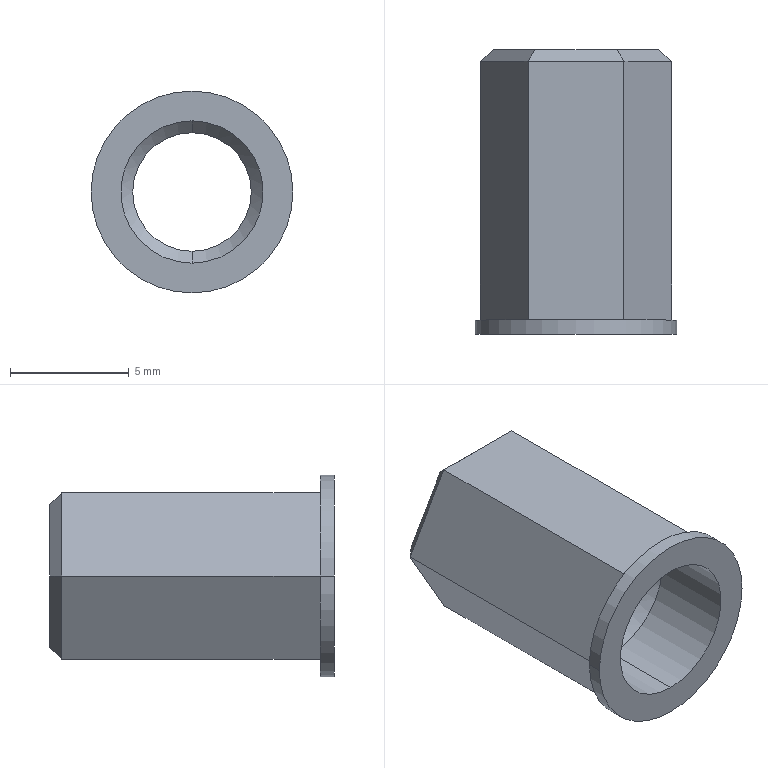Part | SolidWorks | features BaseBody 1 | 1 solid | 23 faces | box 8.5 x 12 x 8.5 mm | volume 246.97 mm3 | plane 15 | cylinder 6 | cone 2 | commonest cylinder face diameters 5 x2 6 x2 8.5 x2
STEP:
#1=CARTESIAN_POINT('',(0.,0.,-3.));
#2=VERTEX_POINT('',#1);
#3=CARTESIAN_POINT('',(0.,0.,3.));
#4=VERTEX_POINT('',#3);
#5=CARTESIAN_POINT('',(0.,0.,0.));
#6=DIRECTION('',(0.,-1.,0.));
#7=DIRECTION('',(0.,0.,-1.));
#8=AXIS2_PLACEMENT_3D('',#5,#6,#7);
#9=CIRCLE('',#8,3.);
#10=EDGE_CURVE('',#2,#4,#9,.T.);
#11=ORIENTED_EDGE('',*,*,#10,.F.);
#12=CARTESIAN_POINT('',(0.,0.,0.));
#13=DIRECTION('',(0.,-1.,0.));
#14=DIRECTION('',(0.,0.,1.));
#15=AXIS2_PLACEMENT_3D('',#12,#13,#14);
#16=CIRCLE('',#15,3.);
#17=EDGE_CURVE('',#4,#2,#16,.T.);
#18=ORIENTED_EDGE('',*,*,#17,.F.);
#19=EDGE_LOOP('',(#11,#18));
#20=FACE_BOUND('',#19,.T.);
#21=CARTESIAN_POINT('',(4.25,0.,0.));
#22=VERTEX_POINT('',#21);
#23=CARTESIAN_POINT('',(-4.25,0.,0.));
#24=VERTEX_POINT('',#23);
#25=CARTESIAN_POINT('',(0.,0.,0.));
#26=DIRECTION('',(0.,-1.,0.));
#27=DIRECTION('',(1.,0.,0.));
#28=AXIS2_PLACEMENT_3D('',#25,#26,#27);
#29=CIRCLE('',#28,4.25);
#30=EDGE_CURVE('',#22,#24,#29,.T.);
#31=ORIENTED_EDGE('',*,*,#30,.T.);
#32=CARTESIAN_POINT('',(0.,0.,0.));
#33=DIRECTION('',(0.,-1.,0.));
#34=DIRECTION('',(-1.,0.,0.));
#35=AXIS2_PLACEMENT_3D('',#32,#33,#34);
#36=CIRCLE('',#35,4.25);
#37=EDGE_CURVE('',#24,#22,#36,.T.);
#38=ORIENTED_EDGE('',*,*,#37,.T.);
#39=EDGE_LOOP('',(#31,#38));
#40=FACE_OUTER_BOUND('',#39,.T.);
#41=CARTESIAN_POINT('',(0.,0.,0.));
#42=DIRECTION('',(0.,1.,0.));
#43=DIRECTION('',(1.,0.,0.));
#44=AXIS2_PLACEMENT_3D('',#41,#42,#43);
#45=PLANE('',#44);
#46=ADVANCED_FACE('',(#20,#40),#45,.F.);
#47=CARTESIAN_POINT('',(-4.25,0.6,0.));
#48=VERTEX_POINT('',#47);
#49=CARTESIAN_POINT('',(-4.25,0.,0.));
#50=DIRECTION('',(0.,1.,0.));
#51=VECTOR('',#50,1000.);
#52=LINE('',#49,#51);
#53=EDGE_CURVE('',#24,#48,#52,.T.);
#54=ORIENTED_EDGE('',*,*,#53,.T.);
#55=CARTESIAN_POINT('',(4.25,0.6,0.));
#56=VERTEX_POINT('',#55);
#57=CARTESIAN_POINT('',(0.,0.6,0.));
#58=DIRECTION('',(0.,-1.,0.));
#59=DIRECTION('',(-1.,0.,0.));
#60=AXIS2_PLACEMENT_3D('',#57,#58,#59);
#61=CIRCLE('',#60,4.25);
#62=EDGE_CURVE('',#48,#56,#61,.T.);
#63=ORIENTED_EDGE('',*,*,#62,.T.);
#64=CARTESIAN_POINT('',(4.25,0.,0.));
#65=DIRECTION('',(0.,1.,0.));
#66=VECTOR('',#65,1000.);
#67=LINE('',#64,#66);
#68=EDGE_CURVE('',#22,#56,#67,.T.);
#69=ORIENTED_EDGE('',*,*,#68,.F.);
#70=ORIENTED_EDGE('',*,*,#37,.F.);
#71=EDGE_LOOP('',(#54,#63,#69,#70));
#72=FACE_OUTER_BOUND('',#71,.T.);
#73=CARTESIAN_POINT('',(0.,0.,0.));
#74=DIRECTION('',(0.,-1.,0.));
#75=DIRECTION('',(-1.,0.,0.));
#76=AXIS2_PLACEMENT_3D('',#73,#74,#75);
#77=CYLINDRICAL_SURFACE('',#76,4.25);
#78=ADVANCED_FACE('',(#72),#77,.T.);
#79=ORIENTED_EDGE('',*,*,#68,.T.);
#80=CARTESIAN_POINT('',(0.,0.6,0.));
#81=DIRECTION('',(0.,-1.,0.));
#82=DIRECTION('',(1.,0.,0.));
#83=AXIS2_PLACEMENT_3D('',#80,#81,#82);
#84=CIRCLE('',#83,4.25);
#85=EDGE_CURVE('',#56,#48,#84,.T.);
#86=ORIENTED_EDGE('',*,*,#85,.T.);
#87=ORIENTED_EDGE('',*,*,#53,.F.);
#88=ORIENTED_EDGE('',*,*,#30,.F.);
#89=EDGE_LOOP('',(#79,#86,#87,#88));
#90=FACE_OUTER_BOUND('',#89,.T.);
#91=CARTESIAN_POINT('',(0.,0.,0.));
#92=DIRECTION('',(0.,-1.,0.));
#93=DIRECTION('',(-1.,0.,0.));
#94=AXIS2_PLACEMENT_3D('',#91,#92,#93);
#95=CYLINDRICAL_SURFACE('',#94,4.25);
#96=ADVANCED_FACE('',(#90),#95,.T.);
#97=CARTESIAN_POINT('',(2.021,0.6,-3.5));
#98=VERTEX_POINT('',#97);
#99=CARTESIAN_POINT('',(-2.021,0.6,-3.5));
#100=VERTEX_POINT('',#99);
#101=CARTESIAN_POINT('',(2.021,0.6,-3.5));
#102=DIRECTION('',(-1.,0.,0.));
#103=VECTOR('',#102,1000.);
#104=LINE('',#101,#103);
#105=EDGE_CURVE('',#98,#100,#104,.T.);
#106=ORIENTED_EDGE('',*,*,#105,.F.);
#107=CARTESIAN_POINT('',(4.041,0.6,0.));
#108=VERTEX_POINT('',#107);
#109=CARTESIAN_POINT('',(4.041,0.6,0.));
#110=DIRECTION('',(-0.5,0.,-0.866));
#111=VECTOR('',#110,1000.);
#112=LINE('',#109,#111);
#113=EDGE_CURVE('',#108,#98,#112,.T.);
#114=ORIENTED_EDGE('',*,*,#113,.F.);
#115=CARTESIAN_POINT('',(2.021,0.6,3.5));
#116=VERTEX_POINT('',#115);
#117=CARTESIAN_POINT('',(2.021,0.6,3.5));
#118=DIRECTION('',(0.5,0.,-0.866));
#119=VECTOR('',#118,1000.);
#120=LINE('',#117,#119);
#121=EDGE_CURVE('',#116,#108,#120,.T.);
#122=ORIENTED_EDGE('',*,*,#121,.F.);
#123=CARTESIAN_POINT('',(-2.021,0.6,3.5));
#124=VERTEX_POINT('',#123);
#125=CARTESIAN_POINT('',(-2.021,0.6,3.5));
#126=DIRECTION('',(1.,0.,0.));
#127=VECTOR('',#126,1000.);
#128=LINE('',#125,#127);
#129=EDGE_CURVE('',#124,#116,#128,.T.);
#130=ORIENTED_EDGE('',*,*,#129,.F.);
#131=CARTESIAN_POINT('',(-4.041,0.6,0.));
#132=VERTEX_POINT('',#131);
#133=CARTESIAN_POINT('',(-4.041,0.6,0.));
#134=DIRECTION('',(0.5,0.,0.866));
#135=VECTOR('',#134,1000.);
#136=LINE('',#133,#135);
#137=EDGE_CURVE('',#132,#124,#136,.T.);
#138=ORIENTED_EDGE('',*,*,#137,.F.);
#139=CARTESIAN_POINT('',(-2.021,0.6,-3.5));
#140=DIRECTION('',(-0.5,0.,0.866));
#141=VECTOR('',#140,1000.);
#142=LINE('',#139,#141);
#143=EDGE_CURVE('',#100,#132,#142,.T.);
#144=ORIENTED_EDGE('',*,*,#143,.F.);
#145=EDGE_LOOP('',(#106,#114,#122,#130,#138,#144));
#146=FACE_BOUND('',#145,.T.);
#147=ORIENTED_EDGE('',*,*,#85,.F.);
#148=ORIENTED_EDGE('',*,*,#62,.F.);
#149=EDGE_LOOP('',(#147,#148));
#150=FACE_OUTER_BOUND('',#149,.T.);
#151=CARTESIAN_POINT('',(0.,0.6,0.));
#152=DIRECTION('',(0.,-1.,0.));
#153=DIRECTION('',(0.,0.,-1.));
#154=AXIS2_PLACEMENT_3D('',#151,#152,#153);
#155=PLANE('',#154);
#156=ADVANCED_FACE('',(#146,#150),#155,.F.);
#157=CARTESIAN_POINT('',(-4.041,11.5,0.));
#158=VERTEX_POINT('',#157);
#159=CARTESIAN_POINT('',(-4.041,0.6,0.));
#160=DIRECTION('',(0.,1.,0.));
#161=VECTOR('',#160,1000.);
#162=LINE('',#159,#161);
#163=EDGE_CURVE('',#132,#158,#162,.T.);
#164=ORIENTED_EDGE('',*,*,#163,.T.);
#165=CARTESIAN_POINT('',(-2.021,11.5,-3.5));
#166=VERTEX_POINT('',#165);
#167=CARTESIAN_POINT('',(-2.021,11.5,-3.5));
#168=DIRECTION('',(-0.5,0.,0.866));
#169=VECTOR('',#168,1000.);
#170=LINE('',#167,#169);
#171=EDGE_CURVE('',#166,#158,#170,.T.);
#172=ORIENTED_EDGE('',*,*,#171,.F.);
#173=CARTESIAN_POINT('',(-2.021,0.6,-3.5));
#174=DIRECTION('',(0.,1.,0.));
#175=VECTOR('',#174,1000.);
#176=LINE('',#173,#175);
#177=EDGE_CURVE('',#100,#166,#176,.T.);
#178=ORIENTED_EDGE('',*,*,#177,.F.);
#179=ORIENTED_EDGE('',*,*,#143,.T.);
#180=EDGE_LOOP('',(#164,#172,#178,#179));
#181=FACE_OUTER_BOUND('',#180,.T.);
#182=CARTESIAN_POINT('',(-2.021,0.,-3.5));
#183=DIRECTION('',(-0.866,0.,-0.5));
#184=DIRECTION('',(-0.5,0.,0.866));
#185=AXIS2_PLACEMENT_3D('',#182,#183,#184);
#186=PLANE('',#185);
#187=ADVANCED_FACE('',(#181),#186,.T.);
#188=ORIENTED_EDGE('',*,*,#177,.T.);
#189=CARTESIAN_POINT('',(2.021,11.5,-3.5));
#190=VERTEX_POINT('',#189);
#191=CARTESIAN_POINT('',(2.021,11.5,-3.5));
#192=DIRECTION('',(-1.,0.,0.));
#193=VECTOR('',#192,1000.);
#194=LINE('',#191,#193);
#195=EDGE_CURVE('',#190,#166,#194,.T.);
#196=ORIENTED_EDGE('',*,*,#195,.F.);
#197=CARTESIAN_POINT('',(2.021,0.6,-3.5));
#198=DIRECTION('',(0.,1.,0.));
#199=VECTOR('',#198,1000.);
#200=LINE('',#197,#199);
#201=EDGE_CURVE('',#98,#190,#200,.T.);
#202=ORIENTED_EDGE('',*,*,#201,.F.);
#203=ORIENTED_EDGE('',*,*,#105,.T.);
#204=EDGE_LOOP('',(#188,#196,#202,#203));
#205=FACE_OUTER_BOUND('',#204,.T.);
#206=CARTESIAN_POINT('',(2.021,0.,-3.5));
#207=DIRECTION('',(0.,0.,-1.));
#208=DIRECTION('',(0.,-1.,0.));
#209=AXIS2_PLACEMENT_3D('',#206,#207,#208);
#210=PLANE('',#209);
#211=ADVANCED_FACE('',(#205),#210,.T.);
#212=ORIENTED_EDGE('',*,*,#201,.T.);
#213=CARTESIAN_POINT('',(4.041,11.5,0.));
#214=VERTEX_POINT('',#213);
#215=CARTESIAN_POINT('',(4.041,11.5,0.));
#216=DIRECTION('',(-0.5,0.,-0.866));
#217=VECTOR('',#216,1000.);
#218=LINE('',#215,#217);
#219=EDGE_CURVE('',#214,#190,#218,.T.);
#220=ORIENTED_EDGE('',*,*,#219,.F.);
#221=CARTESIAN_POINT('',(4.041,0.6,0.));
#222=DIRECTION('',(0.,1.,0.));
#223=VECTOR('',#222,1000.);
#224=LINE('',#221,#223);
#225=EDGE_CURVE('',#108,#214,#224,.T.);
#226=ORIENTED_EDGE('',*,*,#225,.F.);
#227=ORIENTED_EDGE('',*,*,#113,.T.);
#228=EDGE_LOOP('',(#212,#220,#226,#227));
#229=FACE_OUTER_BOUND('',#228,.T.);
#230=CARTESIAN_POINT('',(4.041,0.,0.));
#231=DIRECTION('',(0.866,0.,-0.5));
#232=DIRECTION('',(0.,-1.,0.));
#233=AXIS2_PLACEMENT_3D('',#230,#231,#232);
#234=PLANE('',#233);
#235=ADVANCED_FACE('',(#229),#234,.T.);
#236=ORIENTED_EDGE('',*,*,#225,.T.);
#237=CARTESIAN_POINT('',(2.021,11.5,3.5));
#238=VERTEX_POINT('',#237);
#239=CARTESIAN_POINT('',(2.021,11.5,3.5));
#240=DIRECTION('',(0.5,0.,-0.866));
#241=VECTOR('',#240,1000.);
#242=LINE('',#239,#241);
#243=EDGE_CURVE('',#238,#214,#242,.T.);
#244=ORIENTED_EDGE('',*,*,#243,.F.);
#245=CARTESIAN_POINT('',(2.021,0.6,3.5));
#246=DIRECTION('',(0.,1.,0.));
#247=VECTOR('',#246,1000.);
#248=LINE('',#245,#247);
#249=EDGE_CURVE('',#116,#238,#248,.T.);
#250=ORIENTED_EDGE('',*,*,#249,.F.);
#251=ORIENTED_EDGE('',*,*,#121,.T.);
#252=EDGE_LOOP('',(#236,#244,#250,#251));
#253=FACE_OUTER_BOUND('',#252,.T.);
#254=CARTESIAN_POINT('',(2.021,0.,3.5));
#255=DIRECTION('',(0.866,0.,0.5));
#256=DIRECTION('',(0.,-1.,0.));
#257=AXIS2_PLACEMENT_3D('',#254,#255,#256);
#258=PLANE('',#257);
#259=ADVANCED_FACE('',(#253),#258,.T.);
#260=ORIENTED_EDGE('',*,*,#249,.T.);
#261=CARTESIAN_POINT('',(-2.021,11.5,3.5));
#262=VERTEX_POINT('',#261);
#263=CARTESIAN_POINT('',(-2.021,11.5,3.5));
#264=DIRECTION('',(1.,0.,0.));
#265=VECTOR('',#264,1000.);
#266=LINE('',#263,#265);
#267=EDGE_CURVE('',#262,#238,#266,.T.);
#268=ORIENTED_EDGE('',*,*,#267,.F.);
#269=CARTESIAN_POINT('',(-2.021,0.6,3.5));
#270=DIRECTION('',(0.,1.,0.));
#271=VECTOR('',#270,1000.);
#272=LINE('',#269,#271);
#273=EDGE_CURVE('',#124,#262,#272,.T.);
#274=ORIENTED_EDGE('',*,*,#273,.F.);
#275=ORIENTED_EDGE('',*,*,#129,.T.);
#276=EDGE_LOOP('',(#260,#268,#274,#275));
#277=FACE_OUTER_BOUND('',#276,.T.);
#278=CARTESIAN_POINT('',(-2.021,0.,3.5));
#279=DIRECTION('',(0.,0.,1.));
#280=DIRECTION('',(1.,0.,0.));
#281=AXIS2_PLACEMENT_3D('',#278,#279,#280);
#282=PLANE('',#281);
#283=ADVANCED_FACE('',(#277),#282,.T.);
#284=ORIENTED_EDGE('',*,*,#273,.T.);
#285=CARTESIAN_POINT('',(-4.041,11.5,0.));
#286=DIRECTION('',(0.5,0.,0.866));
#287=VECTOR('',#286,1000.);
#288=LINE('',#285,#287);
#289=EDGE_CURVE('',#158,#262,#288,.T.);
#290=ORIENTED_EDGE('',*,*,#289,.F.);
#291=ORIENTED_EDGE('',*,*,#163,.F.);
#292=ORIENTED_EDGE('',*,*,#137,.T.);
#293=EDGE_LOOP('',(#284,#290,#291,#292));
#294=FACE_OUTER_BOUND('',#293,.T.);
#295=CARTESIAN_POINT('',(-4.041,0.,0.));
#296=DIRECTION('',(-0.866,0.,0.5));
#297=DIRECTION('',(0.,1.,0.));
#298=AXIS2_PLACEMENT_3D('',#295,#296,#297);
#299=PLANE('',#298);
#300=ADVANCED_FACE('',(#294),#299,.T.);
#301=CARTESIAN_POINT('',(-1.732,12.,3.));
#302=VERTEX_POINT('',#301);
#303=CARTESIAN_POINT('',(-2.021,11.5,3.5));
#304=DIRECTION('',(0.378,0.6547,-0.6547));
#305=VECTOR('',#304,1000.);
#306=LINE('',#303,#305);
#307=EDGE_CURVE('',#262,#302,#306,.T.);
#308=ORIENTED_EDGE('',*,*,#307,.T.);
#309=CARTESIAN_POINT('',(-3.464,12.,0.));
#310=VERTEX_POINT('',#309);
#311=CARTESIAN_POINT('',(-3.464,12.,0.));
#312=DIRECTION('',(0.5,0.,0.866));
#313=VECTOR('',#312,1000.);
#314=LINE('',#311,#313);
#315=EDGE_CURVE('',#310,#302,#314,.T.);
#316=ORIENTED_EDGE('',*,*,#315,.F.);
#317=CARTESIAN_POINT('',(-4.041,11.5,0.));
#318=DIRECTION('',(0.7559,0.6547,0.));
#319=VECTOR('',#318,1000.);
#320=LINE('',#317,#319);
#321=EDGE_CURVE('',#158,#310,#320,.T.);
#322=ORIENTED_EDGE('',*,*,#321,.F.);
#323=ORIENTED_EDGE('',*,*,#289,.T.);
#324=EDGE_LOOP('',(#308,#316,#322,#323));
#325=FACE_OUTER_BOUND('',#324,.T.);
#326=CARTESIAN_POINT('',(-2.815,11.75,1.625));
#327=DIRECTION('',(-0.6124,0.7071,0.3536));
#328=DIRECTION('',(0.5,0.,0.866));
#329=AXIS2_PLACEMENT_3D('',#326,#327,#328);
#330=PLANE('',#329);
#331=ADVANCED_FACE('',(#325),#330,.T.);
#332=ORIENTED_EDGE('',*,*,#321,.T.);
#333=CARTESIAN_POINT('',(-1.732,12.,-3.));
#334=VERTEX_POINT('',#333);
#335=CARTESIAN_POINT('',(-1.732,12.,-3.));
#336=DIRECTION('',(-0.5,0.,0.866));
#337=VECTOR('',#336,1000.);
#338=LINE('',#335,#337);
#339=EDGE_CURVE('',#334,#310,#338,.T.);
#340=ORIENTED_EDGE('',*,*,#339,.F.);
#341=CARTESIAN_POINT('',(-2.021,11.5,-3.5));
#342=DIRECTION('',(0.378,0.6547,0.6547));
#343=VECTOR('',#342,1000.);
#344=LINE('',#341,#343);
#345=EDGE_CURVE('',#166,#334,#344,.T.);
#346=ORIENTED_EDGE('',*,*,#345,.F.);
#347=ORIENTED_EDGE('',*,*,#171,.T.);
#348=EDGE_LOOP('',(#332,#340,#346,#347));
#349=FACE_OUTER_BOUND('',#348,.T.);
#350=CARTESIAN_POINT('',(-2.815,11.75,-1.625));
#351=DIRECTION('',(-0.6124,0.7071,-0.3536));
#352=DIRECTION('',(-0.5,0.,0.866));
#353=AXIS2_PLACEMENT_3D('',#350,#351,#352);
#354=PLANE('',#353);
#355=ADVANCED_FACE('',(#349),#354,.T.);
#356=CARTESIAN_POINT('',(1.732,12.,-3.));
#357=VERTEX_POINT('',#356);
#358=CARTESIAN_POINT('',(2.021,11.5,-3.5));
#359=DIRECTION('',(-0.378,0.6547,0.6547));
#360=VECTOR('',#359,1000.);
#361=LINE('',#358,#360);
#362=EDGE_CURVE('',#190,#357,#361,.T.);
#363=ORIENTED_EDGE('',*,*,#362,.F.);
#364=ORIENTED_EDGE('',*,*,#195,.T.);
#365=ORIENTED_EDGE('',*,*,#345,.T.);
#366=CARTESIAN_POINT('',(1.732,12.,-3.));
#367=DIRECTION('',(-1.,0.,0.));
#368=VECTOR('',#367,1000.);
#369=LINE('',#366,#368);
#370=EDGE_CURVE('',#357,#334,#369,.T.);
#371=ORIENTED_EDGE('',*,*,#370,.F.);
#372=EDGE_LOOP('',(#363,#364,#365,#371));
#373=FACE_OUTER_BOUND('',#372,.T.);
#374=CARTESIAN_POINT('',(0.,11.75,-3.25));
#375=DIRECTION('',(0.,0.7071,-0.7071));
#376=DIRECTION('',(-1.,0.,0.));
#377=AXIS2_PLACEMENT_3D('',#374,#375,#376);
#378=PLANE('',#377);
#379=ADVANCED_FACE('',(#373),#378,.T.);
#380=CARTESIAN_POINT('',(-2.5,12.,0.));
#381=VERTEX_POINT('',#380);
#382=CARTESIAN_POINT('',(2.5,12.,0.));
#383=VERTEX_POINT('',#382);
#384=CARTESIAN_POINT('',(0.,12.,0.));
#385=DIRECTION('',(0.,-1.,0.));
#386=DIRECTION('',(-1.,0.,0.));
#387=AXIS2_PLACEMENT_3D('',#384,#385,#386);
#388=CIRCLE('',#387,2.5);
#389=EDGE_CURVE('',#381,#383,#388,.T.);
#390=ORIENTED_EDGE('',*,*,#389,.T.);
#391=CARTESIAN_POINT('',(0.,12.,0.));
#392=DIRECTION('',(0.,-1.,0.));
#393=DIRECTION('',(1.,0.,0.));
#394=AXIS2_PLACEMENT_3D('',#391,#392,#393);
#395=CIRCLE('',#394,2.5);
#396=EDGE_CURVE('',#383,#381,#395,.T.);
#397=ORIENTED_EDGE('',*,*,#396,.T.);
#398=EDGE_LOOP('',(#390,#397));
#399=FACE_BOUND('',#398,.T.);
#400=ORIENTED_EDGE('',*,*,#370,.T.);
#401=ORIENTED_EDGE('',*,*,#339,.T.);
#402=ORIENTED_EDGE('',*,*,#315,.T.);
#403=CARTESIAN_POINT('',(1.732,12.,3.));
#404=VERTEX_POINT('',#403);
#405=CARTESIAN_POINT('',(-1.732,12.,3.));
#406=DIRECTION('',(1.,0.,0.));
#407=VECTOR('',#406,1000.);
#408=LINE('',#405,#407);
#409=EDGE_CURVE('',#302,#404,#408,.T.);
#410=ORIENTED_EDGE('',*,*,#409,.T.);
#411=CARTESIAN_POINT('',(3.464,12.,0.));
#412=VERTEX_POINT('',#411);
#413=CARTESIAN_POINT('',(1.732,12.,3.));
#414=DIRECTION('',(0.5,0.,-0.866));
#415=VECTOR('',#414,1000.);
#416=LINE('',#413,#415);
#417=EDGE_CURVE('',#404,#412,#416,.T.);
#418=ORIENTED_EDGE('',*,*,#417,.T.);
#419=CARTESIAN_POINT('',(3.464,12.,0.));
#420=DIRECTION('',(-0.5,0.,-0.866));
#421=VECTOR('',#420,1000.);
#422=LINE('',#419,#421);
#423=EDGE_CURVE('',#412,#357,#422,.T.);
#424=ORIENTED_EDGE('',*,*,#423,.T.);
#425=EDGE_LOOP('',(#400,#401,#402,#410,#418,#424));
#426=FACE_OUTER_BOUND('',#425,.T.);
#427=CARTESIAN_POINT('',(0.,12.,0.));
#428=DIRECTION('',(0.,1.,0.));
#429=DIRECTION('',(1.,0.,0.));
#430=AXIS2_PLACEMENT_3D('',#427,#428,#429);
#431=PLANE('',#430);
#432=ADVANCED_FACE('',(#399,#426),#431,.T.);
#433=CARTESIAN_POINT('',(-2.5,4.,0.));
#434=VERTEX_POINT('',#433);
#435=CARTESIAN_POINT('',(0.,4.,2.5));
#436=VERTEX_POINT('',#435);
#437=CARTESIAN_POINT('',(0.,4.,0.));
#438=DIRECTION('',(0.,1.,0.));
#439=DIRECTION('',(-1.,0.,0.));
#440=AXIS2_PLACEMENT_3D('',#437,#438,#439);
#441=CIRCLE('',#440,2.5);
#442=EDGE_CURVE('',#434,#436,#441,.T.);
#443=ORIENTED_EDGE('',*,*,#442,.F.);
#444=CARTESIAN_POINT('',(-2.5,4.,0.));
#445=DIRECTION('',(0.,1.,0.));
#446=VECTOR('',#445,1000.);
#447=LINE('',#444,#446);
#448=EDGE_CURVE('',#434,#381,#447,.T.);
#449=ORIENTED_EDGE('',*,*,#448,.T.);
#450=ORIENTED_EDGE('',*,*,#396,.F.);
#451=CARTESIAN_POINT('',(2.5,4.,0.));
#452=VERTEX_POINT('',#451);
#453=CARTESIAN_POINT('',(2.5,4.,0.));
#454=DIRECTION('',(0.,1.,0.));
#455=VECTOR('',#454,1000.);
#456=LINE('',#453,#455);
#457=EDGE_CURVE('',#452,#383,#456,.T.);
#458=ORIENTED_EDGE('',*,*,#457,.F.);
#459=CARTESIAN_POINT('',(0.,4.,0.));
#460=DIRECTION('',(0.,1.,0.));
#461=DIRECTION('',(0.,0.,1.));
#462=AXIS2_PLACEMENT_3D('',#459,#460,#461);
#463=CIRCLE('',#462,2.5);
#464=EDGE_CURVE('',#436,#452,#463,.T.);
#465=ORIENTED_EDGE('',*,*,#464,.F.);
#466=EDGE_LOOP('',(#443,#449,#450,#458,#465));
#467=FACE_OUTER_BOUND('',#466,.T.);
#468=CARTESIAN_POINT('',(0.,0.,0.));
#469=DIRECTION('',(0.,1.,0.));
#470=DIRECTION('',(1.,0.,0.));
#471=AXIS2_PLACEMENT_3D('',#468,#469,#470);
#472=CYLINDRICAL_SURFACE('',#471,2.5);
#473=ADVANCED_FACE('',(#467),#472,.F.);
#474=CARTESIAN_POINT('',(0.,4.,-2.5));
#475=VERTEX_POINT('',#474);
#476=CARTESIAN_POINT('',(0.,3.5,-3.));
#477=VERTEX_POINT('',#476);
#478=CARTESIAN_POINT('',(0.,4.,-2.5));
#479=DIRECTION('',(0.,-0.7071,-0.7071));
#480=VECTOR('',#479,1000.);
#481=LINE('',#478,#480);
#482=EDGE_CURVE('',#475,#477,#481,.T.);
#483=ORIENTED_EDGE('',*,*,#482,.T.);
#484=CARTESIAN_POINT('',(0.,3.5,3.));
#485=VERTEX_POINT('',#484);
#486=CARTESIAN_POINT('',(0.,3.5,0.));
#487=DIRECTION('',(0.,1.,0.));
#488=DIRECTION('',(0.,0.,1.));
#489=AXIS2_PLACEMENT_3D('',#486,#487,#488);
#490=CIRCLE('',#489,3.);
#491=EDGE_CURVE('',#485,#477,#490,.T.);
#492=ORIENTED_EDGE('',*,*,#491,.F.);
#493=CARTESIAN_POINT('',(0.,4.,2.5));
#494=DIRECTION('',(0.,-0.7071,0.7071));
#495=VECTOR('',#494,1000.);
#496=LINE('',#493,#495);
#497=EDGE_CURVE('',#436,#485,#496,.T.);
#498=ORIENTED_EDGE('',*,*,#497,.F.);
#499=ORIENTED_EDGE('',*,*,#464,.T.);
#500=CARTESIAN_POINT('',(0.,4.,0.));
#501=DIRECTION('',(0.,1.,0.));
#502=DIRECTION('',(1.,0.,0.));
#503=AXIS2_PLACEMENT_3D('',#500,#501,#502);
#504=CIRCLE('',#503,2.5);
#505=EDGE_CURVE('',#452,#475,#504,.T.);
#506=ORIENTED_EDGE('',*,*,#505,.T.);
#507=EDGE_LOOP('',(#483,#492,#498,#499,#506));
#508=FACE_OUTER_BOUND('',#507,.T.);
#509=CARTESIAN_POINT('',(0.,3.75,0.));
#510=DIRECTION('',(0.,-1.,0.));
#511=DIRECTION('',(0.,0.,-1.));
#512=AXIS2_PLACEMENT_3D('',#509,#510,#511);
#513=CONICAL_SURFACE('',#512,2.75,0.7854);
#514=ADVANCED_FACE('',(#508),#513,.F.);
#515=ORIENTED_EDGE('',*,*,#457,.T.);
#516=ORIENTED_EDGE('',*,*,#389,.F.);
#517=ORIENTED_EDGE('',*,*,#448,.F.);
#518=CARTESIAN_POINT('',(0.,4.,0.));
#519=DIRECTION('',(0.,1.,0.));
#520=DIRECTION('',(0.,0.,-1.));
#521=AXIS2_PLACEMENT_3D('',#518,#519,#520);
#522=CIRCLE('',#521,2.5);
#523=EDGE_CURVE('',#475,#434,#522,.T.);
#524=ORIENTED_EDGE('',*,*,#523,.F.);
#525=ORIENTED_EDGE('',*,*,#505,.F.);
#526=EDGE_LOOP('',(#515,#516,#517,#524,#525));
#527=FACE_OUTER_BOUND('',#526,.T.);
#528=CARTESIAN_POINT('',(0.,0.,0.));
#529=DIRECTION('',(0.,1.,0.));
#530=DIRECTION('',(1.,0.,0.));
#531=AXIS2_PLACEMENT_3D('',#528,#529,#530);
#532=CYLINDRICAL_SURFACE('',#531,2.5);
#533=ADVANCED_FACE('',(#527),#532,.F.);
#534=ORIENTED_EDGE('',*,*,#497,.T.);
#535=CARTESIAN_POINT('',(0.,3.5,0.));
#536=DIRECTION('',(0.,1.,0.));
#537=DIRECTION('',(0.,0.,-1.));
#538=AXIS2_PLACEMENT_3D('',#535,#536,#537);
#539=CIRCLE('',#538,3.);
#540=EDGE_CURVE('',#477,#485,#539,.T.);
#541=ORIENTED_EDGE('',*,*,#540,.F.);
#542=ORIENTED_EDGE('',*,*,#482,.F.);
#543=ORIENTED_EDGE('',*,*,#523,.T.);
#544=ORIENTED_EDGE('',*,*,#442,.T.);
#545=EDGE_LOOP('',(#534,#541,#542,#543,#544));
#546=FACE_OUTER_BOUND('',#545,.T.);
#547=CARTESIAN_POINT('',(0.,3.75,0.));
#548=DIRECTION('',(0.,-1.,0.));
#549=DIRECTION('',(0.,0.,-1.));
#550=AXIS2_PLACEMENT_3D('',#547,#548,#549);
#551=CONICAL_SURFACE('',#550,2.75,0.7854);
#552=ADVANCED_FACE('',(#546),#551,.F.);
#553=CARTESIAN_POINT('',(0.,0.,3.));
#554=DIRECTION('',(0.,1.,0.));
#555=VECTOR('',#554,1000.);
#556=LINE('',#553,#555);
#557=EDGE_CURVE('',#4,#485,#556,.T.);
#558=ORIENTED_EDGE('',*,*,#557,.F.);
#559=ORIENTED_EDGE('',*,*,#17,.T.);
#560=CARTESIAN_POINT('',(0.,0.,-3.));
#561=DIRECTION('',(0.,1.,0.));
#562=VECTOR('',#561,1000.);
#563=LINE('',#560,#562);
#564=EDGE_CURVE('',#2,#477,#563,.T.);
#565=ORIENTED_EDGE('',*,*,#564,.T.);
#566=ORIENTED_EDGE('',*,*,#540,.T.);
#567=EDGE_LOOP('',(#558,#559,#565,#566));
#568=FACE_OUTER_BOUND('',#567,.T.);
#569=CARTESIAN_POINT('',(0.,0.,0.));
#570=DIRECTION('',(0.,-1.,0.));
#571=DIRECTION('',(0.,0.,1.));
#572=AXIS2_PLACEMENT_3D('',#569,#570,#571);
#573=CYLINDRICAL_SURFACE('',#572,3.);
#574=ADVANCED_FACE('',(#568),#573,.F.);
#575=ORIENTED_EDGE('',*,*,#564,.F.);
#576=ORIENTED_EDGE('',*,*,#10,.T.);
#577=ORIENTED_EDGE('',*,*,#557,.T.);
#578=ORIENTED_EDGE('',*,*,#491,.T.);
#579=EDGE_LOOP('',(#575,#576,#577,#578));
#580=FACE_OUTER_BOUND('',#579,.T.);
#581=CARTESIAN_POINT('',(0.,0.,0.));
#582=DIRECTION('',(0.,-1.,0.));
#583=DIRECTION('',(0.,0.,1.));
#584=AXIS2_PLACEMENT_3D('',#581,#582,#583);
#585=CYLINDRICAL_SURFACE('',#584,3.);
#586=ADVANCED_FACE('',(#580),#585,.F.);
#587=ORIENTED_EDGE('',*,*,#362,.T.);
#588=ORIENTED_EDGE('',*,*,#423,.F.);
#589=CARTESIAN_POINT('',(4.041,11.5,0.));
#590=DIRECTION('',(-0.7559,0.6547,0.));
#591=VECTOR('',#590,1000.);
#592=LINE('',#589,#591);
#593=EDGE_CURVE('',#214,#412,#592,.T.);
#594=ORIENTED_EDGE('',*,*,#593,.F.);
#595=ORIENTED_EDGE('',*,*,#219,.T.);
#596=EDGE_LOOP('',(#587,#588,#594,#595));
#597=FACE_OUTER_BOUND('',#596,.T.);
#598=CARTESIAN_POINT('',(2.815,11.75,-1.625));
#599=DIRECTION('',(0.6124,0.7071,-0.3536));
#600=DIRECTION('',(-0.5,0.,-0.866));
#601=AXIS2_PLACEMENT_3D('',#598,#599,#600);
#602=PLANE('',#601);
#603=ADVANCED_FACE('',(#597),#602,.T.);
#604=ORIENTED_EDGE('',*,*,#593,.T.);
#605=ORIENTED_EDGE('',*,*,#417,.F.);
#606=CARTESIAN_POINT('',(2.021,11.5,3.5));
#607=DIRECTION('',(-0.378,0.6547,-0.6547));
#608=VECTOR('',#607,1000.);
#609=LINE('',#606,#608);
#610=EDGE_CURVE('',#238,#404,#609,.T.);
#611=ORIENTED_EDGE('',*,*,#610,.F.);
#612=ORIENTED_EDGE('',*,*,#243,.T.);
#613=EDGE_LOOP('',(#604,#605,#611,#612));
#614=FACE_OUTER_BOUND('',#613,.T.);
#615=CARTESIAN_POINT('',(2.815,11.75,1.625));
#616=DIRECTION('',(0.6124,0.7071,0.3536));
#617=DIRECTION('',(0.5,0.,-0.866));
#618=AXIS2_PLACEMENT_3D('',#615,#616,#617);
#619=PLANE('',#618);
#620=ADVANCED_FACE('',(#614),#619,.T.);
#621=ORIENTED_EDGE('',*,*,#610,.T.);
#622=ORIENTED_EDGE('',*,*,#409,.F.);
#623=ORIENTED_EDGE('',*,*,#307,.F.);
#624=ORIENTED_EDGE('',*,*,#267,.T.);
#625=EDGE_LOOP('',(#621,#622,#623,#624));
#626=FACE_OUTER_BOUND('',#625,.T.);
#627=CARTESIAN_POINT('',(0.,11.75,3.25));
#628=DIRECTION('',(0.,0.7071,0.7071));
#629=DIRECTION('',(1.,0.,0.));
#630=AXIS2_PLACEMENT_3D('',#627,#628,#629);
#631=PLANE('',#630);
#632=ADVANCED_FACE('',(#626),#631,.T.);
#633=CLOSED_SHELL('',(#46,#78,#96,#156,#187,#211,#235,#259,#283,#300,#331,#355,#379,#432,#473,#514,#533,#552,#574,#586,#603,#620,#632));
#634=MANIFOLD_SOLID_BREP('',#633);
#635=CARTESIAN_POINT('',(0.,0.,0.));
#636=DIRECTION('',(0.,0.,1.));
#637=DIRECTION('',(1.,0.,0.));
#638=AXIS2_PLACEMENT_3D('',#635,#636,#637);
#639=(LENGTH_UNIT()NAMED_UNIT(*)SI_UNIT(.MILLI.,.METRE.));
#640=UNCERTAINTY_MEASURE_WITH_UNIT(LENGTH_MEASURE(0.00001),#639,'','');
#641=(NAMED_UNIT(*)PLANE_ANGLE_UNIT()SI_UNIT($,.RADIAN.));
#642=(NAMED_UNIT(*)SI_UNIT($,.STERADIAN.)SOLID_ANGLE_UNIT());
#643=(GEOMETRIC_REPRESENTATION_CONTEXT(3)GLOBAL_UNCERTAINTY_ASSIGNED_CONTEXT((#640))GLOBAL_UNIT_ASSIGNED_CONTEXT((#639,#641,#642))REPRESENTATION_CONTEXT('',''));
#644=ADVANCED_BREP_SHAPE_REPRESENTATION('',(#634,#638),#643);